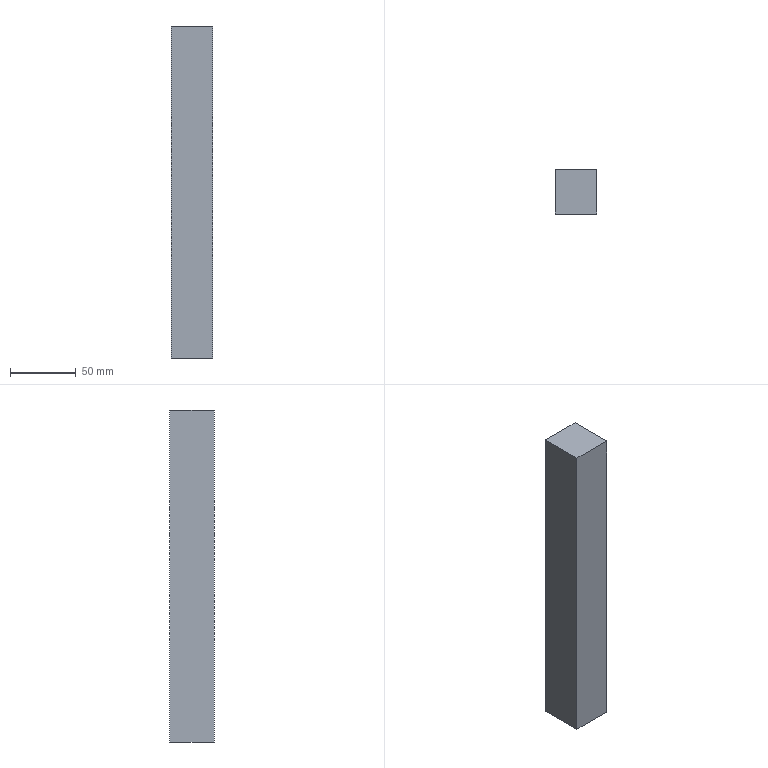Part | SolidWorks | features Extrusion 1 | 1 solid | 6 faces | box 32 x 34 x 253 mm | volume 275264 mm3 | plane 6
STEP:
#1=CARTESIAN_POINT('',(16.,-17.,0.));
#2=VERTEX_POINT('',#1);
#3=CARTESIAN_POINT('',(16.,17.,0.));
#4=VERTEX_POINT('',#3);
#5=CARTESIAN_POINT('',(16.,-17.,0.));
#6=DIRECTION('',(0.,1.,0.));
#7=VECTOR('',#6,1000.);
#8=LINE('',#5,#7);
#9=EDGE_CURVE('',#2,#4,#8,.T.);
#10=ORIENTED_EDGE('',*,*,#9,.T.);
#11=CARTESIAN_POINT('',(16.,17.,253.));
#12=VERTEX_POINT('',#11);
#13=CARTESIAN_POINT('',(16.,17.,253.));
#14=DIRECTION('',(0.,0.,-1.));
#15=VECTOR('',#14,1000.);
#16=LINE('',#13,#15);
#17=EDGE_CURVE('',#12,#4,#16,.T.);
#18=ORIENTED_EDGE('',*,*,#17,.F.);
#19=CARTESIAN_POINT('',(16.,-17.,253.));
#20=VERTEX_POINT('',#19);
#21=CARTESIAN_POINT('',(16.,-17.,253.));
#22=DIRECTION('',(0.,1.,0.));
#23=VECTOR('',#22,1000.);
#24=LINE('',#21,#23);
#25=EDGE_CURVE('',#20,#12,#24,.T.);
#26=ORIENTED_EDGE('',*,*,#25,.F.);
#27=CARTESIAN_POINT('',(16.,-17.,253.));
#28=DIRECTION('',(0.,0.,-1.));
#29=VECTOR('',#28,1000.);
#30=LINE('',#27,#29);
#31=EDGE_CURVE('',#20,#2,#30,.T.);
#32=ORIENTED_EDGE('',*,*,#31,.T.);
#33=EDGE_LOOP('',(#10,#18,#26,#32));
#34=FACE_OUTER_BOUND('',#33,.T.);
#35=CARTESIAN_POINT('',(16.,-17.,253.));
#36=DIRECTION('',(-1.,0.,0.));
#37=DIRECTION('',(0.,0.,1.));
#38=AXIS2_PLACEMENT_3D('',#35,#36,#37);
#39=PLANE('',#38);
#40=ADVANCED_FACE('',(#34),#39,.F.);
#41=CARTESIAN_POINT('',(-16.,17.,0.));
#42=VERTEX_POINT('',#41);
#43=CARTESIAN_POINT('',(-16.,17.,0.));
#44=DIRECTION('',(-1.,0.,0.));
#45=VECTOR('',#44,1000.);
#46=LINE('',#43,#45);
#47=EDGE_CURVE('',#4,#42,#46,.T.);
#48=ORIENTED_EDGE('',*,*,#47,.T.);
#49=CARTESIAN_POINT('',(-16.,17.,253.));
#50=VERTEX_POINT('',#49);
#51=CARTESIAN_POINT('',(-16.,17.,253.));
#52=DIRECTION('',(0.,0.,-1.));
#53=VECTOR('',#52,1000.);
#54=LINE('',#51,#53);
#55=EDGE_CURVE('',#50,#42,#54,.T.);
#56=ORIENTED_EDGE('',*,*,#55,.F.);
#57=CARTESIAN_POINT('',(-16.,17.,253.));
#58=DIRECTION('',(-1.,0.,0.));
#59=VECTOR('',#58,1000.);
#60=LINE('',#57,#59);
#61=EDGE_CURVE('',#12,#50,#60,.T.);
#62=ORIENTED_EDGE('',*,*,#61,.F.);
#63=ORIENTED_EDGE('',*,*,#17,.T.);
#64=EDGE_LOOP('',(#48,#56,#62,#63));
#65=FACE_OUTER_BOUND('',#64,.T.);
#66=CARTESIAN_POINT('',(-16.,17.,253.));
#67=DIRECTION('',(0.,-1.,0.));
#68=DIRECTION('',(0.,0.,-1.));
#69=AXIS2_PLACEMENT_3D('',#66,#67,#68);
#70=PLANE('',#69);
#71=ADVANCED_FACE('',(#65),#70,.F.);
#72=CARTESIAN_POINT('',(-16.,-17.,0.));
#73=VERTEX_POINT('',#72);
#74=CARTESIAN_POINT('',(-16.,-17.,0.));
#75=DIRECTION('',(0.,-1.,0.));
#76=VECTOR('',#75,1000.);
#77=LINE('',#74,#76);
#78=EDGE_CURVE('',#42,#73,#77,.T.);
#79=ORIENTED_EDGE('',*,*,#78,.T.);
#80=CARTESIAN_POINT('',(-16.,-17.,253.));
#81=VERTEX_POINT('',#80);
#82=CARTESIAN_POINT('',(-16.,-17.,253.));
#83=DIRECTION('',(0.,0.,-1.));
#84=VECTOR('',#83,1000.);
#85=LINE('',#82,#84);
#86=EDGE_CURVE('',#81,#73,#85,.T.);
#87=ORIENTED_EDGE('',*,*,#86,.F.);
#88=CARTESIAN_POINT('',(-16.,-17.,253.));
#89=DIRECTION('',(0.,-1.,0.));
#90=VECTOR('',#89,1000.);
#91=LINE('',#88,#90);
#92=EDGE_CURVE('',#50,#81,#91,.T.);
#93=ORIENTED_EDGE('',*,*,#92,.F.);
#94=ORIENTED_EDGE('',*,*,#55,.T.);
#95=EDGE_LOOP('',(#79,#87,#93,#94));
#96=FACE_OUTER_BOUND('',#95,.T.);
#97=CARTESIAN_POINT('',(-16.,-17.,253.));
#98=DIRECTION('',(1.,0.,0.));
#99=DIRECTION('',(0.,0.,-1.));
#100=AXIS2_PLACEMENT_3D('',#97,#98,#99);
#101=PLANE('',#100);
#102=ADVANCED_FACE('',(#96),#101,.F.);
#103=CARTESIAN_POINT('',(-16.,-17.,0.));
#104=DIRECTION('',(1.,0.,0.));
#105=VECTOR('',#104,1000.);
#106=LINE('',#103,#105);
#107=EDGE_CURVE('',#73,#2,#106,.T.);
#108=ORIENTED_EDGE('',*,*,#107,.T.);
#109=ORIENTED_EDGE('',*,*,#31,.F.);
#110=CARTESIAN_POINT('',(-16.,-17.,253.));
#111=DIRECTION('',(1.,0.,0.));
#112=VECTOR('',#111,1000.);
#113=LINE('',#110,#112);
#114=EDGE_CURVE('',#81,#20,#113,.T.);
#115=ORIENTED_EDGE('',*,*,#114,.F.);
#116=ORIENTED_EDGE('',*,*,#86,.T.);
#117=EDGE_LOOP('',(#108,#109,#115,#116));
#118=FACE_OUTER_BOUND('',#117,.T.);
#119=CARTESIAN_POINT('',(-16.,-17.,253.));
#120=DIRECTION('',(0.,1.,0.));
#121=DIRECTION('',(0.,0.,1.));
#122=AXIS2_PLACEMENT_3D('',#119,#120,#121);
#123=PLANE('',#122);
#124=ADVANCED_FACE('',(#118),#123,.F.);
#125=ORIENTED_EDGE('',*,*,#25,.T.);
#126=ORIENTED_EDGE('',*,*,#61,.T.);
#127=ORIENTED_EDGE('',*,*,#92,.T.);
#128=ORIENTED_EDGE('',*,*,#114,.T.);
#129=EDGE_LOOP('',(#125,#126,#127,#128));
#130=FACE_OUTER_BOUND('',#129,.T.);
#131=CARTESIAN_POINT('',(0.,0.,253.));
#132=DIRECTION('',(0.,0.,-1.));
#133=DIRECTION('',(-1.,0.,0.));
#134=AXIS2_PLACEMENT_3D('',#131,#132,#133);
#135=PLANE('',#134);
#136=ADVANCED_FACE('',(#130),#135,.F.);
#137=ORIENTED_EDGE('',*,*,#9,.F.);
#138=ORIENTED_EDGE('',*,*,#107,.F.);
#139=ORIENTED_EDGE('',*,*,#78,.F.);
#140=ORIENTED_EDGE('',*,*,#47,.F.);
#141=EDGE_LOOP('',(#137,#138,#139,#140));
#142=FACE_OUTER_BOUND('',#141,.T.);
#143=CARTESIAN_POINT('',(0.,0.,0.));
#144=DIRECTION('',(0.,0.,-1.));
#145=DIRECTION('',(-1.,0.,0.));
#146=AXIS2_PLACEMENT_3D('',#143,#144,#145);
#147=PLANE('',#146);
#148=ADVANCED_FACE('',(#142),#147,.T.);
#149=CLOSED_SHELL('',(#40,#71,#102,#124,#136,#148));
#150=MANIFOLD_SOLID_BREP('',#149);
#151=CARTESIAN_POINT('',(0.,0.,0.));
#152=DIRECTION('',(0.,0.,1.));
#153=DIRECTION('',(1.,0.,0.));
#154=AXIS2_PLACEMENT_3D('',#151,#152,#153);
#155=(LENGTH_UNIT()NAMED_UNIT(*)SI_UNIT(.MILLI.,.METRE.));
#156=UNCERTAINTY_MEASURE_WITH_UNIT(LENGTH_MEASURE(0.00001),#155,'','');
#157=(NAMED_UNIT(*)PLANE_ANGLE_UNIT()SI_UNIT($,.RADIAN.));
#158=(NAMED_UNIT(*)SI_UNIT($,.STERADIAN.)SOLID_ANGLE_UNIT());
#159=(GEOMETRIC_REPRESENTATION_CONTEXT(3)GLOBAL_UNCERTAINTY_ASSIGNED_CONTEXT((#156))GLOBAL_UNIT_ASSIGNED_CONTEXT((#155,#157,#158))REPRESENTATION_CONTEXT('',''));
#160=ADVANCED_BREP_SHAPE_REPRESENTATION('',(#150,#154),#159);